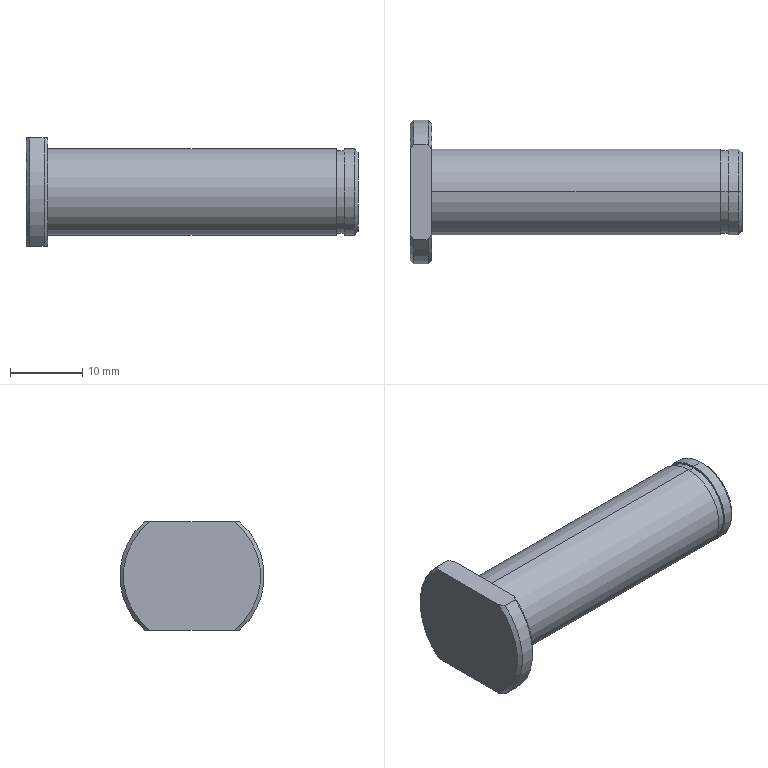Part | STEP file | Roll shaft support bearing shaft | 1 solid | 21 faces | box 46 x 20 x 15 mm | volume 5646 mm3 | cylinder 8 | plane 7 | cone 6 | commonest cylinder face diameters 12 x4 11.5 x2 20 x2